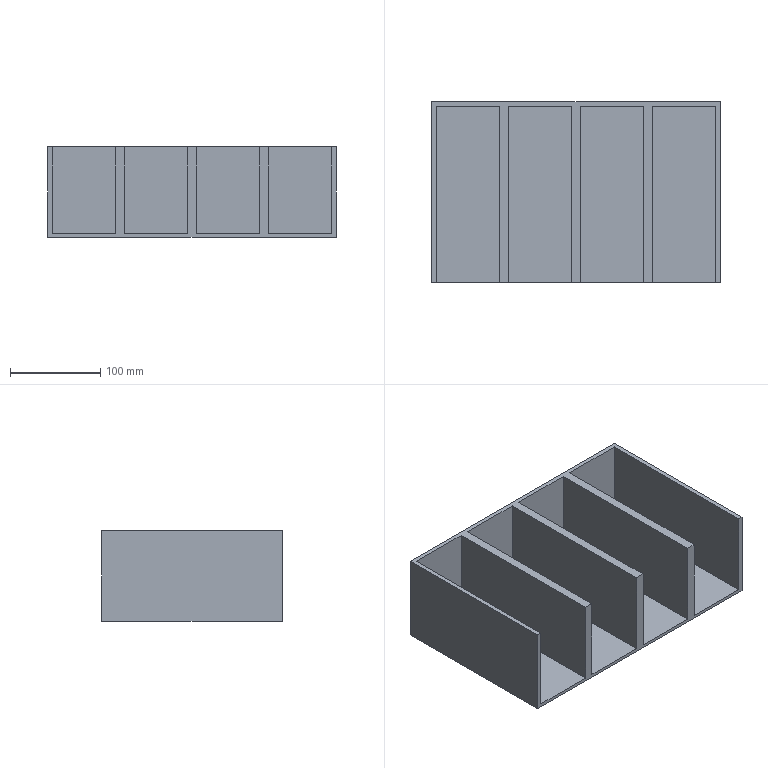Part | STEP file | B1-028 | 1 solid | 22 faces | box 320 x 200 x 100 mm | volume 1158400 mm3 | plane 22